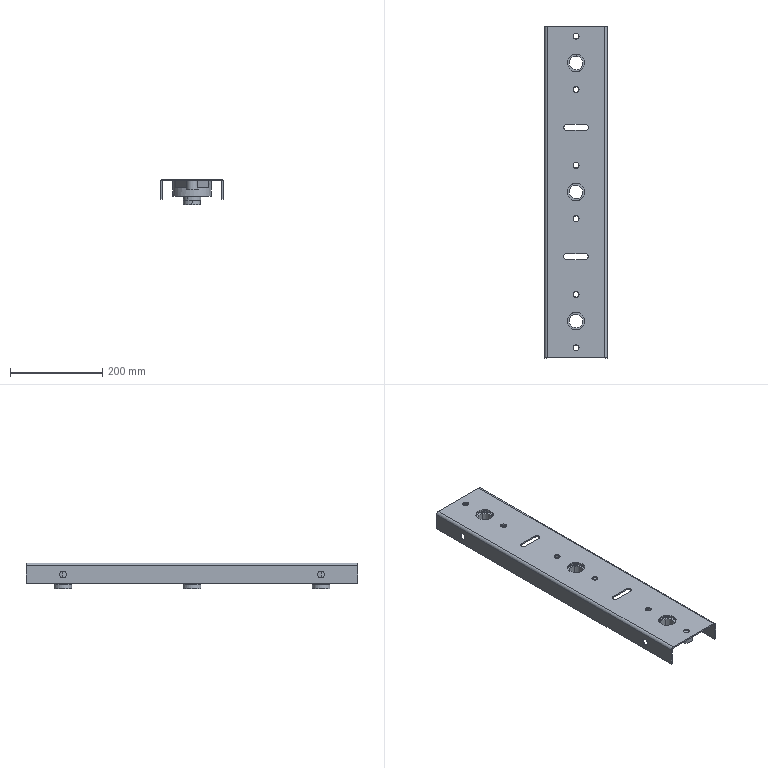Part | SolidWorks | features LayoutProfileFeature 1 | 10 solids | 320 faces | box 136 x 720 x 55.5 mm | volume 917800 mm3 | cylinder 129 | plane 101 | spline 90 | commonest cylinder face diameters 38 x24 13 x18 12 x14 15 x14 30 x12 58 x12